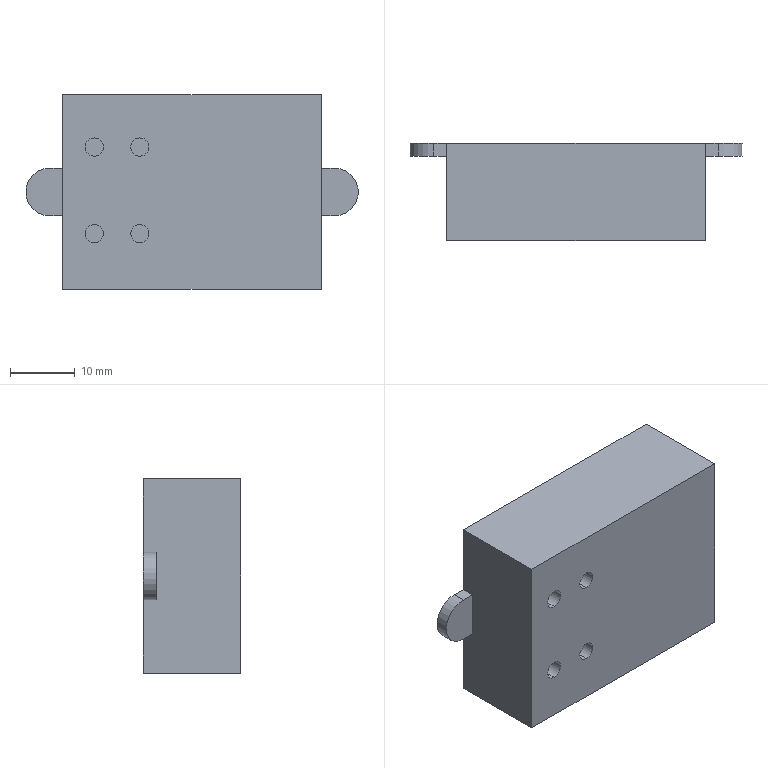Part | SolidWorks | features ICE 2, Extrusion 1 | 1 solid | 26 faces | box 51.375 x 15 x 30 mm | volume 18020 mm3 | plane 16 | cylinder 10 | commonest cylinder face diameters 2.818 x8 7.383 x2
STEP:
#1=CARTESIAN_POINT('',(-8.072,5.,8.36));
#2=VERTEX_POINT('',#1);
#3=CARTESIAN_POINT('',(-8.072,5.,5.542));
#4=VERTEX_POINT('',#3);
#5=CARTESIAN_POINT('',(-8.072,5.,6.951));
#6=DIRECTION('',(0.,-1.,0.));
#7=DIRECTION('',(0.,0.,-1.));
#8=AXIS2_PLACEMENT_3D('',#5,#6,#7);
#9=CIRCLE('',#8,1.409);
#10=EDGE_CURVE('',#2,#4,#9,.T.);
#11=ORIENTED_EDGE('',*,*,#10,.F.);
#12=CARTESIAN_POINT('',(-8.072,0.,8.36));
#13=VERTEX_POINT('',#12);
#14=CARTESIAN_POINT('',(-8.072,5.,8.36));
#15=DIRECTION('',(0.,-1.,0.));
#16=VECTOR('',#15,1000.);
#17=LINE('',#14,#16);
#18=EDGE_CURVE('',#2,#13,#17,.T.);
#19=ORIENTED_EDGE('',*,*,#18,.T.);
#20=CARTESIAN_POINT('',(-8.072,0.,5.542));
#21=VERTEX_POINT('',#20);
#22=CARTESIAN_POINT('',(-8.072,0.,6.951));
#23=DIRECTION('',(0.,-1.,0.));
#24=DIRECTION('',(0.,0.,-1.));
#25=AXIS2_PLACEMENT_3D('',#22,#23,#24);
#26=CIRCLE('',#25,1.409);
#27=EDGE_CURVE('',#13,#21,#26,.T.);
#28=ORIENTED_EDGE('',*,*,#27,.T.);
#29=CARTESIAN_POINT('',(-8.072,5.,5.542));
#30=DIRECTION('',(0.,-1.,0.));
#31=VECTOR('',#30,1000.);
#32=LINE('',#29,#31);
#33=EDGE_CURVE('',#4,#21,#32,.T.);
#34=ORIENTED_EDGE('',*,*,#33,.F.);
#35=EDGE_LOOP('',(#11,#19,#28,#34));
#36=FACE_OUTER_BOUND('',#35,.T.);
#37=CARTESIAN_POINT('',(-8.072,5.,6.951));
#38=DIRECTION('',(0.,-1.,0.));
#39=DIRECTION('',(0.,0.,-1.));
#40=AXIS2_PLACEMENT_3D('',#37,#38,#39);
#41=CYLINDRICAL_SURFACE('',#40,1.409);
#42=ADVANCED_FACE('',(#36),#41,.F.);
#43=CARTESIAN_POINT('',(-15.114,5.,-5.039));
#44=VERTEX_POINT('',#43);
#45=CARTESIAN_POINT('',(-15.114,5.,-7.857));
#46=VERTEX_POINT('',#45);
#47=CARTESIAN_POINT('',(-15.114,5.,-6.448));
#48=DIRECTION('',(0.,-1.,0.));
#49=DIRECTION('',(0.,0.,-1.));
#50=AXIS2_PLACEMENT_3D('',#47,#48,#49);
#51=CIRCLE('',#50,1.409);
#52=EDGE_CURVE('',#44,#46,#51,.T.);
#53=ORIENTED_EDGE('',*,*,#52,.F.);
#54=CARTESIAN_POINT('',(-15.114,0.,-5.039));
#55=VERTEX_POINT('',#54);
#56=CARTESIAN_POINT('',(-15.114,5.,-5.039));
#57=DIRECTION('',(0.,-1.,0.));
#58=VECTOR('',#57,1000.);
#59=LINE('',#56,#58);
#60=EDGE_CURVE('',#44,#55,#59,.T.);
#61=ORIENTED_EDGE('',*,*,#60,.T.);
#62=CARTESIAN_POINT('',(-15.114,0.,-7.857));
#63=VERTEX_POINT('',#62);
#64=CARTESIAN_POINT('',(-15.114,0.,-6.448));
#65=DIRECTION('',(0.,-1.,0.));
#66=DIRECTION('',(0.,0.,-1.));
#67=AXIS2_PLACEMENT_3D('',#64,#65,#66);
#68=CIRCLE('',#67,1.409);
#69=EDGE_CURVE('',#55,#63,#68,.T.);
#70=ORIENTED_EDGE('',*,*,#69,.T.);
#71=CARTESIAN_POINT('',(-15.114,5.,-7.857));
#72=DIRECTION('',(0.,-1.,0.));
#73=VECTOR('',#72,1000.);
#74=LINE('',#71,#73);
#75=EDGE_CURVE('',#46,#63,#74,.T.);
#76=ORIENTED_EDGE('',*,*,#75,.F.);
#77=EDGE_LOOP('',(#53,#61,#70,#76));
#78=FACE_OUTER_BOUND('',#77,.T.);
#79=CARTESIAN_POINT('',(-15.114,5.,-6.448));
#80=DIRECTION('',(0.,-1.,0.));
#81=DIRECTION('',(0.,0.,-1.));
#82=AXIS2_PLACEMENT_3D('',#79,#80,#81);
#83=CYLINDRICAL_SURFACE('',#82,1.409);
#84=ADVANCED_FACE('',(#78),#83,.F.);
#85=CARTESIAN_POINT('',(-8.072,5.,-5.039));
#86=VERTEX_POINT('',#85);
#87=CARTESIAN_POINT('',(-8.072,5.,-7.857));
#88=VERTEX_POINT('',#87);
#89=CARTESIAN_POINT('',(-8.072,5.,-6.448));
#90=DIRECTION('',(0.,-1.,0.));
#91=DIRECTION('',(0.,0.,-1.));
#92=AXIS2_PLACEMENT_3D('',#89,#90,#91);
#93=CIRCLE('',#92,1.409);
#94=EDGE_CURVE('',#86,#88,#93,.T.);
#95=ORIENTED_EDGE('',*,*,#94,.F.);
#96=CARTESIAN_POINT('',(-8.072,0.,-5.039));
#97=VERTEX_POINT('',#96);
#98=CARTESIAN_POINT('',(-8.072,5.,-5.039));
#99=DIRECTION('',(0.,-1.,0.));
#100=VECTOR('',#99,1000.);
#101=LINE('',#98,#100);
#102=EDGE_CURVE('',#86,#97,#101,.T.);
#103=ORIENTED_EDGE('',*,*,#102,.T.);
#104=CARTESIAN_POINT('',(-8.072,0.,-7.857));
#105=VERTEX_POINT('',#104);
#106=CARTESIAN_POINT('',(-8.072,0.,-6.448));
#107=DIRECTION('',(0.,-1.,0.));
#108=DIRECTION('',(0.,0.,-1.));
#109=AXIS2_PLACEMENT_3D('',#106,#107,#108);
#110=CIRCLE('',#109,1.409);
#111=EDGE_CURVE('',#97,#105,#110,.T.);
#112=ORIENTED_EDGE('',*,*,#111,.T.);
#113=CARTESIAN_POINT('',(-8.072,5.,-7.857));
#114=DIRECTION('',(0.,-1.,0.));
#115=VECTOR('',#114,1000.);
#116=LINE('',#113,#115);
#117=EDGE_CURVE('',#88,#105,#116,.T.);
#118=ORIENTED_EDGE('',*,*,#117,.F.);
#119=EDGE_LOOP('',(#95,#103,#112,#118));
#120=FACE_OUTER_BOUND('',#119,.T.);
#121=CARTESIAN_POINT('',(-8.072,5.,-6.448));
#122=DIRECTION('',(0.,-1.,0.));
#123=DIRECTION('',(0.,0.,-1.));
#124=AXIS2_PLACEMENT_3D('',#121,#122,#123);
#125=CYLINDRICAL_SURFACE('',#124,1.409);
#126=ADVANCED_FACE('',(#120),#125,.F.);
#127=CARTESIAN_POINT('',(-15.114,5.,8.36));
#128=VERTEX_POINT('',#127);
#129=CARTESIAN_POINT('',(-15.114,5.,5.542));
#130=VERTEX_POINT('',#129);
#131=CARTESIAN_POINT('',(-15.114,5.,6.951));
#132=DIRECTION('',(0.,-1.,0.));
#133=DIRECTION('',(0.,0.,-1.));
#134=AXIS2_PLACEMENT_3D('',#131,#132,#133);
#135=CIRCLE('',#134,1.409);
#136=EDGE_CURVE('',#128,#130,#135,.T.);
#137=ORIENTED_EDGE('',*,*,#136,.F.);
#138=CARTESIAN_POINT('',(-15.114,0.,8.36));
#139=VERTEX_POINT('',#138);
#140=CARTESIAN_POINT('',(-15.114,5.,8.36));
#141=DIRECTION('',(0.,-1.,0.));
#142=VECTOR('',#141,1000.);
#143=LINE('',#140,#142);
#144=EDGE_CURVE('',#128,#139,#143,.T.);
#145=ORIENTED_EDGE('',*,*,#144,.T.);
#146=CARTESIAN_POINT('',(-15.114,0.,5.542));
#147=VERTEX_POINT('',#146);
#148=CARTESIAN_POINT('',(-15.114,0.,6.951));
#149=DIRECTION('',(0.,-1.,0.));
#150=DIRECTION('',(0.,0.,-1.));
#151=AXIS2_PLACEMENT_3D('',#148,#149,#150);
#152=CIRCLE('',#151,1.409);
#153=EDGE_CURVE('',#139,#147,#152,.T.);
#154=ORIENTED_EDGE('',*,*,#153,.T.);
#155=CARTESIAN_POINT('',(-15.114,5.,5.542));
#156=DIRECTION('',(0.,-1.,0.));
#157=VECTOR('',#156,1000.);
#158=LINE('',#155,#157);
#159=EDGE_CURVE('',#130,#147,#158,.T.);
#160=ORIENTED_EDGE('',*,*,#159,.F.);
#161=EDGE_LOOP('',(#137,#145,#154,#160));
#162=FACE_OUTER_BOUND('',#161,.T.);
#163=CARTESIAN_POINT('',(-15.114,5.,6.951));
#164=DIRECTION('',(0.,-1.,0.));
#165=DIRECTION('',(0.,0.,-1.));
#166=AXIS2_PLACEMENT_3D('',#163,#164,#165);
#167=CYLINDRICAL_SURFACE('',#166,1.409);
#168=ADVANCED_FACE('',(#162),#167,.F.);
#169=CARTESIAN_POINT('',(20.,15.,-3.692));
#170=VERTEX_POINT('',#169);
#171=CARTESIAN_POINT('',(20.,15.,-15.));
#172=VERTEX_POINT('',#171);
#173=CARTESIAN_POINT('',(20.,15.,-15.));
#174=DIRECTION('',(0.,0.,-1.));
#175=VECTOR('',#174,1000.);
#176=LINE('',#173,#175);
#177=EDGE_CURVE('',#170,#172,#176,.T.);
#178=ORIENTED_EDGE('',*,*,#177,.F.);
#179=CARTESIAN_POINT('',(20.,13.,-3.692));
#180=VERTEX_POINT('',#179);
#181=CARTESIAN_POINT('',(20.,15.,-3.692));
#182=DIRECTION('',(0.,-1.,0.));
#183=VECTOR('',#182,1000.);
#184=LINE('',#181,#183);
#185=EDGE_CURVE('',#170,#180,#184,.T.);
#186=ORIENTED_EDGE('',*,*,#185,.T.);
#187=CARTESIAN_POINT('',(20.,13.,3.692));
#188=VERTEX_POINT('',#187);
#189=CARTESIAN_POINT('',(20.,13.,-15.));
#190=DIRECTION('',(0.,0.,-1.));
#191=VECTOR('',#190,1000.);
#192=LINE('',#189,#191);
#193=EDGE_CURVE('',#188,#180,#192,.T.);
#194=ORIENTED_EDGE('',*,*,#193,.F.);
#195=CARTESIAN_POINT('',(20.,15.,3.692));
#196=VERTEX_POINT('',#195);
#197=CARTESIAN_POINT('',(20.,15.,3.692));
#198=DIRECTION('',(0.,1.,0.));
#199=VECTOR('',#198,1000.);
#200=LINE('',#197,#199);
#201=EDGE_CURVE('',#188,#196,#200,.T.);
#202=ORIENTED_EDGE('',*,*,#201,.T.);
#203=CARTESIAN_POINT('',(20.,15.,15.));
#204=VERTEX_POINT('',#203);
#205=CARTESIAN_POINT('',(20.,15.,-15.));
#206=DIRECTION('',(0.,0.,-1.));
#207=VECTOR('',#206,1000.);
#208=LINE('',#205,#207);
#209=EDGE_CURVE('',#204,#196,#208,.T.);
#210=ORIENTED_EDGE('',*,*,#209,.F.);
#211=CARTESIAN_POINT('',(20.,0.,15.));
#212=VERTEX_POINT('',#211);
#213=CARTESIAN_POINT('',(20.,15.,15.));
#214=DIRECTION('',(0.,-1.,0.));
#215=VECTOR('',#214,1000.);
#216=LINE('',#213,#215);
#217=EDGE_CURVE('',#204,#212,#216,.T.);
#218=ORIENTED_EDGE('',*,*,#217,.T.);
#219=CARTESIAN_POINT('',(20.,0.,-15.));
#220=VERTEX_POINT('',#219);
#221=CARTESIAN_POINT('',(20.,0.,-15.));
#222=DIRECTION('',(0.,0.,-1.));
#223=VECTOR('',#222,1000.);
#224=LINE('',#221,#223);
#225=EDGE_CURVE('',#212,#220,#224,.T.);
#226=ORIENTED_EDGE('',*,*,#225,.T.);
#227=CARTESIAN_POINT('',(20.,15.,-15.));
#228=DIRECTION('',(0.,-1.,0.));
#229=VECTOR('',#228,1000.);
#230=LINE('',#227,#229);
#231=EDGE_CURVE('',#172,#220,#230,.T.);
#232=ORIENTED_EDGE('',*,*,#231,.F.);
#233=EDGE_LOOP('',(#178,#186,#194,#202,#210,#218,#226,#232));
#234=FACE_OUTER_BOUND('',#233,.T.);
#235=CARTESIAN_POINT('',(20.,15.,-15.));
#236=DIRECTION('',(-1.,0.,0.));
#237=DIRECTION('',(0.,0.,1.));
#238=AXIS2_PLACEMENT_3D('',#235,#236,#237);
#239=PLANE('',#238);
#240=ADVANCED_FACE('',(#234),#239,.F.);
#241=CARTESIAN_POINT('',(-20.,0.,-15.));
#242=VERTEX_POINT('',#241);
#243=CARTESIAN_POINT('',(-20.,0.,-15.));
#244=DIRECTION('',(-1.,0.,0.));
#245=VECTOR('',#244,1000.);
#246=LINE('',#243,#245);
#247=EDGE_CURVE('',#220,#242,#246,.T.);
#248=ORIENTED_EDGE('',*,*,#247,.T.);
#249=CARTESIAN_POINT('',(-20.,15.,-15.));
#250=VERTEX_POINT('',#249);
#251=CARTESIAN_POINT('',(-20.,15.,-15.));
#252=DIRECTION('',(0.,-1.,0.));
#253=VECTOR('',#252,1000.);
#254=LINE('',#251,#253);
#255=EDGE_CURVE('',#250,#242,#254,.T.);
#256=ORIENTED_EDGE('',*,*,#255,.F.);
#257=CARTESIAN_POINT('',(-20.,15.,-15.));
#258=DIRECTION('',(-1.,0.,0.));
#259=VECTOR('',#258,1000.);
#260=LINE('',#257,#259);
#261=EDGE_CURVE('',#172,#250,#260,.T.);
#262=ORIENTED_EDGE('',*,*,#261,.F.);
#263=ORIENTED_EDGE('',*,*,#231,.T.);
#264=EDGE_LOOP('',(#248,#256,#262,#263));
#265=FACE_OUTER_BOUND('',#264,.T.);
#266=CARTESIAN_POINT('',(-20.,15.,-15.));
#267=DIRECTION('',(0.,0.,1.));
#268=DIRECTION('',(1.,0.,0.));
#269=AXIS2_PLACEMENT_3D('',#266,#267,#268);
#270=PLANE('',#269);
#271=ADVANCED_FACE('',(#265),#270,.F.);
#272=CARTESIAN_POINT('',(-20.,13.,-3.692));
#273=VERTEX_POINT('',#272);
#274=CARTESIAN_POINT('',(-20.,13.,3.692));
#275=VERTEX_POINT('',#274);
#276=CARTESIAN_POINT('',(-20.,13.,-15.));
#277=DIRECTION('',(0.,0.,1.));
#278=VECTOR('',#277,1000.);
#279=LINE('',#276,#278);
#280=EDGE_CURVE('',#273,#275,#279,.T.);
#281=ORIENTED_EDGE('',*,*,#280,.F.);
#282=CARTESIAN_POINT('',(-20.,15.,-3.692));
#283=VERTEX_POINT('',#282);
#284=CARTESIAN_POINT('',(-20.,15.,-3.692));
#285=DIRECTION('',(0.,1.,0.));
#286=VECTOR('',#285,1000.);
#287=LINE('',#284,#286);
#288=EDGE_CURVE('',#273,#283,#287,.T.);
#289=ORIENTED_EDGE('',*,*,#288,.T.);
#290=CARTESIAN_POINT('',(-20.,15.,-15.));
#291=DIRECTION('',(0.,0.,1.));
#292=VECTOR('',#291,1000.);
#293=LINE('',#290,#292);
#294=EDGE_CURVE('',#250,#283,#293,.T.);
#295=ORIENTED_EDGE('',*,*,#294,.F.);
#296=ORIENTED_EDGE('',*,*,#255,.T.);
#297=CARTESIAN_POINT('',(-20.,0.,15.));
#298=VERTEX_POINT('',#297);
#299=CARTESIAN_POINT('',(-20.,0.,-15.));
#300=DIRECTION('',(0.,0.,1.));
#301=VECTOR('',#300,1000.);
#302=LINE('',#299,#301);
#303=EDGE_CURVE('',#242,#298,#302,.T.);
#304=ORIENTED_EDGE('',*,*,#303,.T.);
#305=CARTESIAN_POINT('',(-20.,15.,15.));
#306=VERTEX_POINT('',#305);
#307=CARTESIAN_POINT('',(-20.,15.,15.));
#308=DIRECTION('',(0.,-1.,0.));
#309=VECTOR('',#308,1000.);
#310=LINE('',#307,#309);
#311=EDGE_CURVE('',#306,#298,#310,.T.);
#312=ORIENTED_EDGE('',*,*,#311,.F.);
#313=CARTESIAN_POINT('',(-20.,15.,3.692));
#314=VERTEX_POINT('',#313);
#315=CARTESIAN_POINT('',(-20.,15.,-15.));
#316=DIRECTION('',(0.,0.,1.));
#317=VECTOR('',#316,1000.);
#318=LINE('',#315,#317);
#319=EDGE_CURVE('',#314,#306,#318,.T.);
#320=ORIENTED_EDGE('',*,*,#319,.F.);
#321=CARTESIAN_POINT('',(-20.,15.,3.692));
#322=DIRECTION('',(0.,-1.,0.));
#323=VECTOR('',#322,1000.);
#324=LINE('',#321,#323);
#325=EDGE_CURVE('',#314,#275,#324,.T.);
#326=ORIENTED_EDGE('',*,*,#325,.T.);
#327=EDGE_LOOP('',(#281,#289,#295,#296,#304,#312,#320,#326));
#328=FACE_OUTER_BOUND('',#327,.T.);
#329=CARTESIAN_POINT('',(-20.,15.,-15.));
#330=DIRECTION('',(1.,0.,0.));
#331=DIRECTION('',(0.,0.,-1.));
#332=AXIS2_PLACEMENT_3D('',#329,#330,#331);
#333=PLANE('',#332);
#334=ADVANCED_FACE('',(#328),#333,.F.);
#335=CARTESIAN_POINT('',(-20.,0.,15.));
#336=DIRECTION('',(1.,0.,0.));
#337=VECTOR('',#336,1000.);
#338=LINE('',#335,#337);
#339=EDGE_CURVE('',#298,#212,#338,.T.);
#340=ORIENTED_EDGE('',*,*,#339,.T.);
#341=ORIENTED_EDGE('',*,*,#217,.F.);
#342=CARTESIAN_POINT('',(-20.,15.,15.));
#343=DIRECTION('',(1.,0.,0.));
#344=VECTOR('',#343,1000.);
#345=LINE('',#342,#344);
#346=EDGE_CURVE('',#306,#204,#345,.T.);
#347=ORIENTED_EDGE('',*,*,#346,.F.);
#348=ORIENTED_EDGE('',*,*,#311,.T.);
#349=EDGE_LOOP('',(#340,#341,#347,#348));
#350=FACE_OUTER_BOUND('',#349,.T.);
#351=CARTESIAN_POINT('',(-20.,15.,15.));
#352=DIRECTION('',(0.,0.,-1.));
#353=DIRECTION('',(-1.,0.,0.));
#354=AXIS2_PLACEMENT_3D('',#351,#352,#353);
#355=PLANE('',#354);
#356=ADVANCED_FACE('',(#350),#355,.F.);
#357=ORIENTED_EDGE('',*,*,#209,.T.);
#358=CARTESIAN_POINT('',(21.996,15.,3.692));
#359=VERTEX_POINT('',#358);
#360=CARTESIAN_POINT('',(-21.996,15.,3.692));
#361=DIRECTION('',(1.,0.,0.));
#362=VECTOR('',#361,1000.);
#363=LINE('',#360,#362);
#364=EDGE_CURVE('',#196,#359,#363,.T.);
#365=ORIENTED_EDGE('',*,*,#364,.T.);
#366=CARTESIAN_POINT('',(21.996,15.,-3.692));
#367=VERTEX_POINT('',#366);
#368=CARTESIAN_POINT('',(21.996,15.,0.));
#369=DIRECTION('',(0.,1.,0.));
#370=DIRECTION('',(0.,0.,1.));
#371=AXIS2_PLACEMENT_3D('',#368,#369,#370);
#372=CIRCLE('',#371,3.692);
#373=EDGE_CURVE('',#359,#367,#372,.T.);
#374=ORIENTED_EDGE('',*,*,#373,.T.);
#375=CARTESIAN_POINT('',(-21.996,15.,-3.692));
#376=DIRECTION('',(-1.,0.,0.));
#377=VECTOR('',#376,1000.);
#378=LINE('',#375,#377);
#379=EDGE_CURVE('',#367,#170,#378,.T.);
#380=ORIENTED_EDGE('',*,*,#379,.T.);
#381=ORIENTED_EDGE('',*,*,#177,.T.);
#382=ORIENTED_EDGE('',*,*,#261,.T.);
#383=ORIENTED_EDGE('',*,*,#294,.T.);
#384=CARTESIAN_POINT('',(-21.996,15.,-3.692));
#385=VERTEX_POINT('',#384);
#386=CARTESIAN_POINT('',(-21.996,15.,-3.692));
#387=DIRECTION('',(-1.,0.,0.));
#388=VECTOR('',#387,1000.);
#389=LINE('',#386,#388);
#390=EDGE_CURVE('',#283,#385,#389,.T.);
#391=ORIENTED_EDGE('',*,*,#390,.T.);
#392=CARTESIAN_POINT('',(-21.996,15.,3.692));
#393=VERTEX_POINT('',#392);
#394=CARTESIAN_POINT('',(-21.996,15.,0.));
#395=DIRECTION('',(0.,1.,0.));
#396=DIRECTION('',(0.,0.,1.));
#397=AXIS2_PLACEMENT_3D('',#394,#395,#396);
#398=CIRCLE('',#397,3.692);
#399=EDGE_CURVE('',#385,#393,#398,.T.);
#400=ORIENTED_EDGE('',*,*,#399,.T.);
#401=CARTESIAN_POINT('',(-21.996,15.,3.692));
#402=DIRECTION('',(1.,0.,0.));
#403=VECTOR('',#402,1000.);
#404=LINE('',#401,#403);
#405=EDGE_CURVE('',#393,#314,#404,.T.);
#406=ORIENTED_EDGE('',*,*,#405,.T.);
#407=ORIENTED_EDGE('',*,*,#319,.T.);
#408=ORIENTED_EDGE('',*,*,#346,.T.);
#409=EDGE_LOOP('',(#357,#365,#374,#380,#381,#382,#383,#391,#400,#406,#407,#408));
#410=FACE_OUTER_BOUND('',#409,.T.);
#411=CARTESIAN_POINT('',(0.,15.,0.));
#412=DIRECTION('',(0.,1.,0.));
#413=DIRECTION('',(0.,0.,1.));
#414=AXIS2_PLACEMENT_3D('',#411,#412,#413);
#415=PLANE('',#414);
#416=ADVANCED_FACE('',(#410),#415,.T.);
#417=CARTESIAN_POINT('',(-8.072,0.,6.951));
#418=DIRECTION('',(0.,-1.,0.));
#419=DIRECTION('',(0.,0.,-1.));
#420=AXIS2_PLACEMENT_3D('',#417,#418,#419);
#421=CIRCLE('',#420,1.409);
#422=EDGE_CURVE('',#21,#13,#421,.T.);
#423=ORIENTED_EDGE('',*,*,#422,.F.);
#424=ORIENTED_EDGE('',*,*,#27,.F.);
#425=EDGE_LOOP('',(#423,#424));
#426=FACE_BOUND('',#425,.T.);
#427=CARTESIAN_POINT('',(-15.114,0.,-6.448));
#428=DIRECTION('',(0.,-1.,0.));
#429=DIRECTION('',(0.,0.,-1.));
#430=AXIS2_PLACEMENT_3D('',#427,#428,#429);
#431=CIRCLE('',#430,1.409);
#432=EDGE_CURVE('',#63,#55,#431,.T.);
#433=ORIENTED_EDGE('',*,*,#432,.F.);
#434=ORIENTED_EDGE('',*,*,#69,.F.);
#435=EDGE_LOOP('',(#433,#434));
#436=FACE_BOUND('',#435,.T.);
#437=CARTESIAN_POINT('',(-8.072,0.,-6.448));
#438=DIRECTION('',(0.,-1.,0.));
#439=DIRECTION('',(0.,0.,-1.));
#440=AXIS2_PLACEMENT_3D('',#437,#438,#439);
#441=CIRCLE('',#440,1.409);
#442=EDGE_CURVE('',#105,#97,#441,.T.);
#443=ORIENTED_EDGE('',*,*,#442,.F.);
#444=ORIENTED_EDGE('',*,*,#111,.F.);
#445=EDGE_LOOP('',(#443,#444));
#446=FACE_BOUND('',#445,.T.);
#447=CARTESIAN_POINT('',(-15.114,0.,6.951));
#448=DIRECTION('',(0.,-1.,0.));
#449=DIRECTION('',(0.,0.,-1.));
#450=AXIS2_PLACEMENT_3D('',#447,#448,#449);
#451=CIRCLE('',#450,1.409);
#452=EDGE_CURVE('',#147,#139,#451,.T.);
#453=ORIENTED_EDGE('',*,*,#452,.F.);
#454=ORIENTED_EDGE('',*,*,#153,.F.);
#455=EDGE_LOOP('',(#453,#454));
#456=FACE_BOUND('',#455,.T.);
#457=ORIENTED_EDGE('',*,*,#225,.F.);
#458=ORIENTED_EDGE('',*,*,#339,.F.);
#459=ORIENTED_EDGE('',*,*,#303,.F.);
#460=ORIENTED_EDGE('',*,*,#247,.F.);
#461=EDGE_LOOP('',(#457,#458,#459,#460));
#462=FACE_OUTER_BOUND('',#461,.T.);
#463=CARTESIAN_POINT('',(0.,0.,0.));
#464=DIRECTION('',(0.,1.,0.));
#465=DIRECTION('',(0.,0.,1.));
#466=AXIS2_PLACEMENT_3D('',#463,#464,#465);
#467=PLANE('',#466);
#468=ADVANCED_FACE('',(#426,#436,#446,#456,#462),#467,.F.);
#469=ORIENTED_EDGE('',*,*,#399,.F.);
#470=CARTESIAN_POINT('',(-21.996,13.,-3.692));
#471=VERTEX_POINT('',#470);
#472=CARTESIAN_POINT('',(-21.996,13.,-3.692));
#473=DIRECTION('',(0.,1.,0.));
#474=VECTOR('',#473,1000.);
#475=LINE('',#472,#474);
#476=EDGE_CURVE('',#471,#385,#475,.T.);
#477=ORIENTED_EDGE('',*,*,#476,.F.);
#478=CARTESIAN_POINT('',(-21.996,13.,3.692));
#479=VERTEX_POINT('',#478);
#480=CARTESIAN_POINT('',(-21.996,13.,0.));
#481=DIRECTION('',(0.,1.,0.));
#482=DIRECTION('',(0.,0.,1.));
#483=AXIS2_PLACEMENT_3D('',#480,#481,#482);
#484=CIRCLE('',#483,3.692);
#485=EDGE_CURVE('',#471,#479,#484,.T.);
#486=ORIENTED_EDGE('',*,*,#485,.T.);
#487=CARTESIAN_POINT('',(-21.996,13.,3.692));
#488=DIRECTION('',(0.,1.,0.));
#489=VECTOR('',#488,1000.);
#490=LINE('',#487,#489);
#491=EDGE_CURVE('',#479,#393,#490,.T.);
#492=ORIENTED_EDGE('',*,*,#491,.T.);
#493=EDGE_LOOP('',(#469,#477,#486,#492));
#494=FACE_OUTER_BOUND('',#493,.T.);
#495=CARTESIAN_POINT('',(-21.996,13.,0.));
#496=DIRECTION('',(0.,1.,0.));
#497=DIRECTION('',(0.,0.,1.));
#498=AXIS2_PLACEMENT_3D('',#495,#496,#497);
#499=CYLINDRICAL_SURFACE('',#498,3.692);
#500=ADVANCED_FACE('',(#494),#499,.T.);
#501=CARTESIAN_POINT('',(-21.996,13.,-3.692));
#502=DIRECTION('',(-1.,0.,0.));
#503=VECTOR('',#502,1000.);
#504=LINE('',#501,#503);
#505=EDGE_CURVE('',#273,#471,#504,.T.);
#506=ORIENTED_EDGE('',*,*,#505,.F.);
#507=ORIENTED_EDGE('',*,*,#280,.T.);
#508=CARTESIAN_POINT('',(-21.996,13.,3.692));
#509=DIRECTION('',(1.,0.,0.));
#510=VECTOR('',#509,1000.);
#511=LINE('',#508,#510);
#512=EDGE_CURVE('',#479,#275,#511,.T.);
#513=ORIENTED_EDGE('',*,*,#512,.F.);
#514=ORIENTED_EDGE('',*,*,#485,.F.);
#515=EDGE_LOOP('',(#506,#507,#513,#514));
#516=FACE_OUTER_BOUND('',#515,.T.);
#517=CARTESIAN_POINT('',(-21.996,13.,0.));
#518=DIRECTION('',(0.,1.,0.));
#519=DIRECTION('',(0.,0.,1.));
#520=AXIS2_PLACEMENT_3D('',#517,#518,#519);
#521=PLANE('',#520);
#522=ADVANCED_FACE('',(#516),#521,.F.);
#523=ORIENTED_EDGE('',*,*,#325,.F.);
#524=ORIENTED_EDGE('',*,*,#405,.F.);
#525=ORIENTED_EDGE('',*,*,#491,.F.);
#526=ORIENTED_EDGE('',*,*,#512,.T.);
#527=EDGE_LOOP('',(#523,#524,#525,#526));
#528=FACE_OUTER_BOUND('',#527,.T.);
#529=CARTESIAN_POINT('',(-21.996,13.,3.692));
#530=DIRECTION('',(0.,0.,1.));
#531=DIRECTION('',(1.,0.,0.));
#532=AXIS2_PLACEMENT_3D('',#529,#530,#531);
#533=PLANE('',#532);
#534=ADVANCED_FACE('',(#528),#533,.T.);
#535=ORIENTED_EDGE('',*,*,#288,.F.);
#536=ORIENTED_EDGE('',*,*,#505,.T.);
#537=ORIENTED_EDGE('',*,*,#476,.T.);
#538=ORIENTED_EDGE('',*,*,#390,.F.);
#539=EDGE_LOOP('',(#535,#536,#537,#538));
#540=FACE_OUTER_BOUND('',#539,.T.);
#541=CARTESIAN_POINT('',(-21.996,13.,-3.692));
#542=DIRECTION('',(0.,0.,-1.));
#543=DIRECTION('',(-1.,0.,0.));
#544=AXIS2_PLACEMENT_3D('',#541,#542,#543);
#545=PLANE('',#544);
#546=ADVANCED_FACE('',(#540),#545,.T.);
#547=CARTESIAN_POINT('',(21.996,13.,3.692));
#548=VERTEX_POINT('',#547);
#549=CARTESIAN_POINT('',(-21.996,13.,3.692));
#550=DIRECTION('',(1.,0.,0.));
#551=VECTOR('',#550,1000.);
#552=LINE('',#549,#551);
#553=EDGE_CURVE('',#188,#548,#552,.T.);
#554=ORIENTED_EDGE('',*,*,#553,.F.);
#555=ORIENTED_EDGE('',*,*,#193,.T.);
#556=CARTESIAN_POINT('',(21.996,13.,-3.692));
#557=VERTEX_POINT('',#556);
#558=CARTESIAN_POINT('',(-21.996,13.,-3.692));
#559=DIRECTION('',(-1.,0.,0.));
#560=VECTOR('',#559,1000.);
#561=LINE('',#558,#560);
#562=EDGE_CURVE('',#557,#180,#561,.T.);
#563=ORIENTED_EDGE('',*,*,#562,.F.);
#564=CARTESIAN_POINT('',(21.996,13.,0.));
#565=DIRECTION('',(0.,1.,0.));
#566=DIRECTION('',(0.,0.,1.));
#567=AXIS2_PLACEMENT_3D('',#564,#565,#566);
#568=CIRCLE('',#567,3.692);
#569=EDGE_CURVE('',#548,#557,#568,.T.);
#570=ORIENTED_EDGE('',*,*,#569,.F.);
#571=EDGE_LOOP('',(#554,#555,#563,#570));
#572=FACE_OUTER_BOUND('',#571,.T.);
#573=CARTESIAN_POINT('',(-21.996,13.,0.));
#574=DIRECTION('',(0.,1.,0.));
#575=DIRECTION('',(0.,0.,1.));
#576=AXIS2_PLACEMENT_3D('',#573,#574,#575);
#577=PLANE('',#576);
#578=ADVANCED_FACE('',(#572),#577,.F.);
#579=ORIENTED_EDGE('',*,*,#185,.F.);
#580=ORIENTED_EDGE('',*,*,#379,.F.);
#581=CARTESIAN_POINT('',(21.996,13.,-3.692));
#582=DIRECTION('',(0.,1.,0.));
#583=VECTOR('',#582,1000.);
#584=LINE('',#581,#583);
#585=EDGE_CURVE('',#557,#367,#584,.T.);
#586=ORIENTED_EDGE('',*,*,#585,.F.);
#587=ORIENTED_EDGE('',*,*,#562,.T.);
#588=EDGE_LOOP('',(#579,#580,#586,#587));
#589=FACE_OUTER_BOUND('',#588,.T.);
#590=CARTESIAN_POINT('',(-21.996,13.,-3.692));
#591=DIRECTION('',(0.,0.,-1.));
#592=DIRECTION('',(-1.,0.,0.));
#593=AXIS2_PLACEMENT_3D('',#590,#591,#592);
#594=PLANE('',#593);
#595=ADVANCED_FACE('',(#589),#594,.T.);
#596=ORIENTED_EDGE('',*,*,#201,.F.);
#597=ORIENTED_EDGE('',*,*,#553,.T.);
#598=CARTESIAN_POINT('',(21.996,13.,3.692));
#599=DIRECTION('',(0.,1.,0.));
#600=VECTOR('',#599,1000.);
#601=LINE('',#598,#600);
#602=EDGE_CURVE('',#548,#359,#601,.T.);
#603=ORIENTED_EDGE('',*,*,#602,.T.);
#604=ORIENTED_EDGE('',*,*,#364,.F.);
#605=EDGE_LOOP('',(#596,#597,#603,#604));
#606=FACE_OUTER_BOUND('',#605,.T.);
#607=CARTESIAN_POINT('',(-21.996,13.,3.692));
#608=DIRECTION('',(0.,0.,1.));
#609=DIRECTION('',(1.,0.,0.));
#610=AXIS2_PLACEMENT_3D('',#607,#608,#609);
#611=PLANE('',#610);
#612=ADVANCED_FACE('',(#606),#611,.T.);
#613=ORIENTED_EDGE('',*,*,#373,.F.);
#614=ORIENTED_EDGE('',*,*,#602,.F.);
#615=ORIENTED_EDGE('',*,*,#569,.T.);
#616=ORIENTED_EDGE('',*,*,#585,.T.);
#617=EDGE_LOOP('',(#613,#614,#615,#616));
#618=FACE_OUTER_BOUND('',#617,.T.);
#619=CARTESIAN_POINT('',(21.996,13.,0.));
#620=DIRECTION('',(0.,1.,0.));
#621=DIRECTION('',(0.,0.,1.));
#622=AXIS2_PLACEMENT_3D('',#619,#620,#621);
#623=CYLINDRICAL_SURFACE('',#622,3.692);
#624=ADVANCED_FACE('',(#618),#623,.T.);
#625=ORIENTED_EDGE('',*,*,#144,.F.);
#626=CARTESIAN_POINT('',(-15.114,5.,6.951));
#627=DIRECTION('',(0.,-1.,0.));
#628=DIRECTION('',(0.,0.,-1.));
#629=AXIS2_PLACEMENT_3D('',#626,#627,#628);
#630=CIRCLE('',#629,1.409);
#631=EDGE_CURVE('',#130,#128,#630,.T.);
#632=ORIENTED_EDGE('',*,*,#631,.F.);
#633=ORIENTED_EDGE('',*,*,#159,.T.);
#634=ORIENTED_EDGE('',*,*,#452,.T.);
#635=EDGE_LOOP('',(#625,#632,#633,#634));
#636=FACE_OUTER_BOUND('',#635,.T.);
#637=CARTESIAN_POINT('',(-15.114,5.,6.951));
#638=DIRECTION('',(0.,-1.,0.));
#639=DIRECTION('',(0.,0.,-1.));
#640=AXIS2_PLACEMENT_3D('',#637,#638,#639);
#641=CYLINDRICAL_SURFACE('',#640,1.409);
#642=ADVANCED_FACE('',(#636),#641,.F.);
#643=ORIENTED_EDGE('',*,*,#631,.T.);
#644=ORIENTED_EDGE('',*,*,#136,.T.);
#645=EDGE_LOOP('',(#643,#644));
#646=FACE_OUTER_BOUND('',#645,.T.);
#647=CARTESIAN_POINT('',(-15.114,5.,6.951));
#648=DIRECTION('',(0.,-1.,0.));
#649=DIRECTION('',(0.,0.,-1.));
#650=AXIS2_PLACEMENT_3D('',#647,#648,#649);
#651=PLANE('',#650);
#652=ADVANCED_FACE('',(#646),#651,.T.);
#653=ORIENTED_EDGE('',*,*,#102,.F.);
#654=CARTESIAN_POINT('',(-8.072,5.,-6.448));
#655=DIRECTION('',(0.,-1.,0.));
#656=DIRECTION('',(0.,0.,-1.));
#657=AXIS2_PLACEMENT_3D('',#654,#655,#656);
#658=CIRCLE('',#657,1.409);
#659=EDGE_CURVE('',#88,#86,#658,.T.);
#660=ORIENTED_EDGE('',*,*,#659,.F.);
#661=ORIENTED_EDGE('',*,*,#117,.T.);
#662=ORIENTED_EDGE('',*,*,#442,.T.);
#663=EDGE_LOOP('',(#653,#660,#661,#662));
#664=FACE_OUTER_BOUND('',#663,.T.);
#665=CARTESIAN_POINT('',(-8.072,5.,-6.448));
#666=DIRECTION('',(0.,-1.,0.));
#667=DIRECTION('',(0.,0.,-1.));
#668=AXIS2_PLACEMENT_3D('',#665,#666,#667);
#669=CYLINDRICAL_SURFACE('',#668,1.409);
#670=ADVANCED_FACE('',(#664),#669,.F.);
#671=ORIENTED_EDGE('',*,*,#659,.T.);
#672=ORIENTED_EDGE('',*,*,#94,.T.);
#673=EDGE_LOOP('',(#671,#672));
#674=FACE_OUTER_BOUND('',#673,.T.);
#675=CARTESIAN_POINT('',(-8.072,5.,-6.448));
#676=DIRECTION('',(0.,-1.,0.));
#677=DIRECTION('',(0.,0.,-1.));
#678=AXIS2_PLACEMENT_3D('',#675,#676,#677);
#679=PLANE('',#678);
#680=ADVANCED_FACE('',(#674),#679,.T.);
#681=ORIENTED_EDGE('',*,*,#60,.F.);
#682=CARTESIAN_POINT('',(-15.114,5.,-6.448));
#683=DIRECTION('',(0.,-1.,0.));
#684=DIRECTION('',(0.,0.,-1.));
#685=AXIS2_PLACEMENT_3D('',#682,#683,#684);
#686=CIRCLE('',#685,1.409);
#687=EDGE_CURVE('',#46,#44,#686,.T.);
#688=ORIENTED_EDGE('',*,*,#687,.F.);
#689=ORIENTED_EDGE('',*,*,#75,.T.);
#690=ORIENTED_EDGE('',*,*,#432,.T.);
#691=EDGE_LOOP('',(#681,#688,#689,#690));
#692=FACE_OUTER_BOUND('',#691,.T.);
#693=CARTESIAN_POINT('',(-15.114,5.,-6.448));
#694=DIRECTION('',(0.,-1.,0.));
#695=DIRECTION('',(0.,0.,-1.));
#696=AXIS2_PLACEMENT_3D('',#693,#694,#695);
#697=CYLINDRICAL_SURFACE('',#696,1.409);
#698=ADVANCED_FACE('',(#692),#697,.F.);
#699=ORIENTED_EDGE('',*,*,#687,.T.);
#700=ORIENTED_EDGE('',*,*,#52,.T.);
#701=EDGE_LOOP('',(#699,#700));
#702=FACE_OUTER_BOUND('',#701,.T.);
#703=CARTESIAN_POINT('',(-15.114,5.,-6.448));
#704=DIRECTION('',(0.,-1.,0.));
#705=DIRECTION('',(0.,0.,-1.));
#706=AXIS2_PLACEMENT_3D('',#703,#704,#705);
#707=PLANE('',#706);
#708=ADVANCED_FACE('',(#702),#707,.T.);
#709=ORIENTED_EDGE('',*,*,#18,.F.);
#710=CARTESIAN_POINT('',(-8.072,5.,6.951));
#711=DIRECTION('',(0.,-1.,0.));
#712=DIRECTION('',(0.,0.,-1.));
#713=AXIS2_PLACEMENT_3D('',#710,#711,#712);
#714=CIRCLE('',#713,1.409);
#715=EDGE_CURVE('',#4,#2,#714,.T.);
#716=ORIENTED_EDGE('',*,*,#715,.F.);
#717=ORIENTED_EDGE('',*,*,#33,.T.);
#718=ORIENTED_EDGE('',*,*,#422,.T.);
#719=EDGE_LOOP('',(#709,#716,#717,#718));
#720=FACE_OUTER_BOUND('',#719,.T.);
#721=CARTESIAN_POINT('',(-8.072,5.,6.951));
#722=DIRECTION('',(0.,-1.,0.));
#723=DIRECTION('',(0.,0.,-1.));
#724=AXIS2_PLACEMENT_3D('',#721,#722,#723);
#725=CYLINDRICAL_SURFACE('',#724,1.409);
#726=ADVANCED_FACE('',(#720),#725,.F.);
#727=ORIENTED_EDGE('',*,*,#715,.T.);
#728=ORIENTED_EDGE('',*,*,#10,.T.);
#729=EDGE_LOOP('',(#727,#728));
#730=FACE_OUTER_BOUND('',#729,.T.);
#731=CARTESIAN_POINT('',(-8.072,5.,6.951));
#732=DIRECTION('',(0.,-1.,0.));
#733=DIRECTION('',(0.,0.,-1.));
#734=AXIS2_PLACEMENT_3D('',#731,#732,#733);
#735=PLANE('',#734);
#736=ADVANCED_FACE('',(#730),#735,.T.);
#737=CLOSED_SHELL('',(#42,#84,#126,#168,#240,#271,#334,#356,#416,#468,#500,#522,#534,#546,#578,#595,#612,#624,#642,#652,#670,#680,#698,#708,#726,#736));
#738=MANIFOLD_SOLID_BREP('',#737);
#739=CARTESIAN_POINT('',(0.,0.,0.));
#740=DIRECTION('',(0.,0.,1.));
#741=DIRECTION('',(1.,0.,0.));
#742=AXIS2_PLACEMENT_3D('',#739,#740,#741);
#743=(LENGTH_UNIT()NAMED_UNIT(*)SI_UNIT(.MILLI.,.METRE.));
#744=UNCERTAINTY_MEASURE_WITH_UNIT(LENGTH_MEASURE(0.00001),#743,'','');
#745=(NAMED_UNIT(*)PLANE_ANGLE_UNIT()SI_UNIT($,.RADIAN.));
#746=(NAMED_UNIT(*)SI_UNIT($,.STERADIAN.)SOLID_ANGLE_UNIT());
#747=(GEOMETRIC_REPRESENTATION_CONTEXT(3)GLOBAL_UNCERTAINTY_ASSIGNED_CONTEXT((#744))GLOBAL_UNIT_ASSIGNED_CONTEXT((#743,#745,#746))REPRESENTATION_CONTEXT('',''));
#748=ADVANCED_BREP_SHAPE_REPRESENTATION('',(#738,#742),#747);